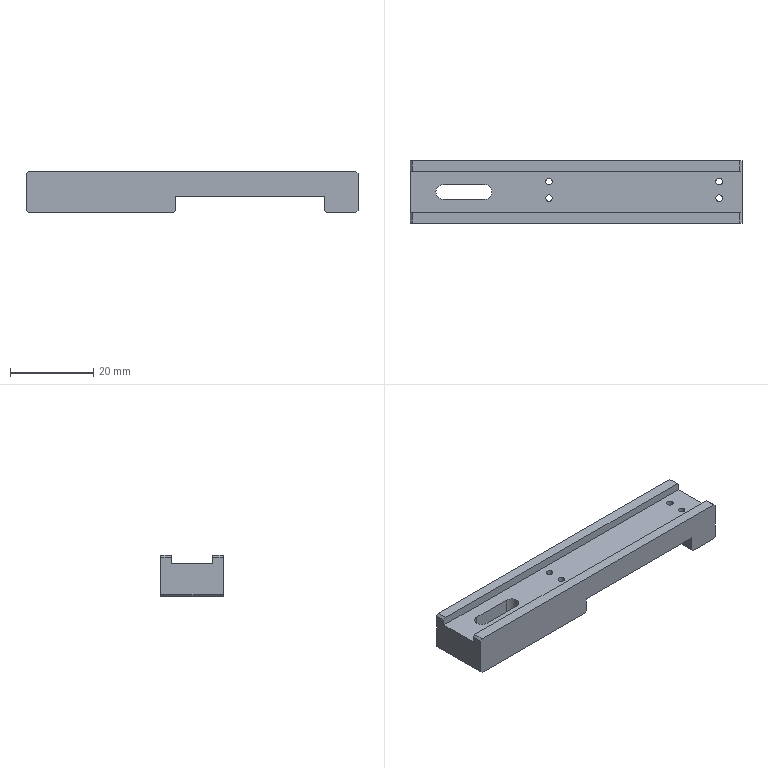Part | NX | 1 solid | 35 faces | box 80 x 15 x 10 mm | volume 7810 mm3 | plane 24 | cylinder 11 | commonest cylinder face diameters 1.6 x8 3.5 x3
STEP:
#1=CARTESIAN_POINT('',(-33.75,0.,-2.));
#2=VERTEX_POINT('',#1);
#3=CARTESIAN_POINT('',(-32.,1.75,-2.));
#4=VERTEX_POINT('',#3);
#5=CARTESIAN_POINT('',(-32.,0.,-2.));
#6=DIRECTION('',(0.,0.,-1.));
#7=DIRECTION('',(-1.,0.,0.));
#8=AXIS2_PLACEMENT_3D('',#5,#6,#7);
#9=CIRCLE('',#8,1.75);
#10=EDGE_CURVE('',#2,#4,#9,.T.);
#11=ORIENTED_EDGE('',*,*,#10,.F.);
#12=CARTESIAN_POINT('',(-33.75,0.,-10.));
#13=VERTEX_POINT('',#12);
#14=CARTESIAN_POINT('',(-33.75,0.,15.));
#15=DIRECTION('',(0.,0.,-1.));
#16=VECTOR('',#15,1000.);
#17=LINE('',#14,#16);
#18=EDGE_CURVE('',#2,#13,#17,.T.);
#19=ORIENTED_EDGE('',*,*,#18,.T.);
#20=CARTESIAN_POINT('',(-32.,1.75,-10.));
#21=VERTEX_POINT('',#20);
#22=CARTESIAN_POINT('',(-32.,0.,-10.));
#23=DIRECTION('',(0.,0.,-1.));
#24=DIRECTION('',(-1.,0.,0.));
#25=AXIS2_PLACEMENT_3D('',#22,#23,#24);
#26=CIRCLE('',#25,1.75);
#27=EDGE_CURVE('',#13,#21,#26,.T.);
#28=ORIENTED_EDGE('',*,*,#27,.T.);
#29=CARTESIAN_POINT('',(-32.,1.75,15.));
#30=DIRECTION('',(0.,0.,-1.));
#31=VECTOR('',#30,1000.);
#32=LINE('',#29,#31);
#33=EDGE_CURVE('',#4,#21,#32,.T.);
#34=ORIENTED_EDGE('',*,*,#33,.F.);
#35=EDGE_LOOP('',(#11,#19,#28,#34));
#36=FACE_BOUND('',#35,.T.);
#37=CARTESIAN_POINT('',(-32.,0.,15.));
#38=DIRECTION('',(0.,0.,-1.));
#39=DIRECTION('',(1.,0.,0.));
#40=AXIS2_PLACEMENT_3D('',#37,#38,#39);
#41=CYLINDRICAL_SURFACE('',#40,1.75);
#42=ADVANCED_FACE('',(#36),#41,.F.);
#43=CARTESIAN_POINT('',(33.7,2.5,-2.));
#44=VERTEX_POINT('',#43);
#45=CARTESIAN_POINT('',(35.3,2.5,-2.));
#46=VERTEX_POINT('',#45);
#47=CARTESIAN_POINT('',(34.5,2.5,-2.));
#48=DIRECTION('',(0.,0.,1.));
#49=DIRECTION('',(-1.,0.,0.));
#50=AXIS2_PLACEMENT_3D('',#47,#48,#49);
#51=CIRCLE('',#50,0.8);
#52=EDGE_CURVE('',#44,#46,#51,.T.);
#53=ORIENTED_EDGE('',*,*,#52,.T.);
#54=CARTESIAN_POINT('',(35.3,2.5,-10.));
#55=VERTEX_POINT('',#54);
#56=CARTESIAN_POINT('',(35.3,2.5,-10.));
#57=DIRECTION('',(0.,0.,-1.));
#58=VECTOR('',#57,1000.);
#59=LINE('',#56,#58);
#60=EDGE_CURVE('',#55,#46,#59,.F.);
#61=ORIENTED_EDGE('',*,*,#60,.F.);
#62=CARTESIAN_POINT('',(33.7,2.5,-10.));
#63=VERTEX_POINT('',#62);
#64=CARTESIAN_POINT('',(34.5,2.5,-10.));
#65=DIRECTION('',(0.,0.,-1.));
#66=DIRECTION('',(-1.,0.,0.));
#67=AXIS2_PLACEMENT_3D('',#64,#65,#66);
#68=CIRCLE('',#67,0.8);
#69=EDGE_CURVE('',#55,#63,#68,.T.);
#70=ORIENTED_EDGE('',*,*,#69,.T.);
#71=CARTESIAN_POINT('',(33.7,2.5,-10.));
#72=DIRECTION('',(0.,0.,-1.));
#73=VECTOR('',#72,1000.);
#74=LINE('',#71,#73);
#75=EDGE_CURVE('',#63,#44,#74,.F.);
#76=ORIENTED_EDGE('',*,*,#75,.T.);
#77=EDGE_LOOP('',(#53,#61,#70,#76));
#78=FACE_BOUND('',#77,.T.);
#79=CARTESIAN_POINT('',(34.5,2.5,-10.));
#80=DIRECTION('',(0.,0.,-1.));
#81=DIRECTION('',(1.,0.,0.));
#82=AXIS2_PLACEMENT_3D('',#79,#80,#81);
#83=CYLINDRICAL_SURFACE('',#82,0.8);
#84=ADVANCED_FACE('',(#78),#83,.F.);
#85=CARTESIAN_POINT('',(33.7,-1.5,-2.));
#86=VERTEX_POINT('',#85);
#87=CARTESIAN_POINT('',(35.3,-1.5,-2.));
#88=VERTEX_POINT('',#87);
#89=CARTESIAN_POINT('',(34.5,-1.5,-2.));
#90=DIRECTION('',(0.,0.,1.));
#91=DIRECTION('',(-1.,0.,0.));
#92=AXIS2_PLACEMENT_3D('',#89,#90,#91);
#93=CIRCLE('',#92,0.8);
#94=EDGE_CURVE('',#86,#88,#93,.T.);
#95=ORIENTED_EDGE('',*,*,#94,.T.);
#96=CARTESIAN_POINT('',(35.3,-1.5,-10.));
#97=VERTEX_POINT('',#96);
#98=CARTESIAN_POINT('',(35.3,-1.5,-10.));
#99=DIRECTION('',(0.,0.,-1.));
#100=VECTOR('',#99,1000.);
#101=LINE('',#98,#100);
#102=EDGE_CURVE('',#97,#88,#101,.F.);
#103=ORIENTED_EDGE('',*,*,#102,.F.);
#104=CARTESIAN_POINT('',(33.7,-1.5,-10.));
#105=VERTEX_POINT('',#104);
#106=CARTESIAN_POINT('',(34.5,-1.5,-10.));
#107=DIRECTION('',(0.,0.,-1.));
#108=DIRECTION('',(-1.,0.,0.));
#109=AXIS2_PLACEMENT_3D('',#106,#107,#108);
#110=CIRCLE('',#109,0.8);
#111=EDGE_CURVE('',#97,#105,#110,.T.);
#112=ORIENTED_EDGE('',*,*,#111,.T.);
#113=CARTESIAN_POINT('',(33.7,-1.5,-10.));
#114=DIRECTION('',(0.,0.,-1.));
#115=VECTOR('',#114,1000.);
#116=LINE('',#113,#115);
#117=EDGE_CURVE('',#105,#86,#116,.F.);
#118=ORIENTED_EDGE('',*,*,#117,.T.);
#119=EDGE_LOOP('',(#95,#103,#112,#118));
#120=FACE_BOUND('',#119,.T.);
#121=CARTESIAN_POINT('',(34.5,-1.5,-10.));
#122=DIRECTION('',(0.,0.,-1.));
#123=DIRECTION('',(1.,0.,0.));
#124=AXIS2_PLACEMENT_3D('',#121,#122,#123);
#125=CYLINDRICAL_SURFACE('',#124,0.8);
#126=ADVANCED_FACE('',(#120),#125,.F.);
#127=CARTESIAN_POINT('',(-7.3,-1.5,-2.));
#128=VERTEX_POINT('',#127);
#129=CARTESIAN_POINT('',(-5.7,-1.5,-2.));
#130=VERTEX_POINT('',#129);
#131=CARTESIAN_POINT('',(-6.5,-1.5,-2.));
#132=DIRECTION('',(0.,0.,1.));
#133=DIRECTION('',(-1.,0.,0.));
#134=AXIS2_PLACEMENT_3D('',#131,#132,#133);
#135=CIRCLE('',#134,0.8);
#136=EDGE_CURVE('',#128,#130,#135,.T.);
#137=ORIENTED_EDGE('',*,*,#136,.T.);
#138=CARTESIAN_POINT('',(-5.7,-1.5,-10.));
#139=VERTEX_POINT('',#138);
#140=CARTESIAN_POINT('',(-5.7,-1.5,-10.));
#141=DIRECTION('',(0.,0.,-1.));
#142=VECTOR('',#141,1000.);
#143=LINE('',#140,#142);
#144=EDGE_CURVE('',#139,#130,#143,.F.);
#145=ORIENTED_EDGE('',*,*,#144,.F.);
#146=CARTESIAN_POINT('',(-7.3,-1.5,-10.));
#147=VERTEX_POINT('',#146);
#148=CARTESIAN_POINT('',(-6.5,-1.5,-10.));
#149=DIRECTION('',(0.,0.,-1.));
#150=DIRECTION('',(-1.,0.,0.));
#151=AXIS2_PLACEMENT_3D('',#148,#149,#150);
#152=CIRCLE('',#151,0.8);
#153=EDGE_CURVE('',#139,#147,#152,.T.);
#154=ORIENTED_EDGE('',*,*,#153,.T.);
#155=CARTESIAN_POINT('',(-7.3,-1.5,-10.));
#156=DIRECTION('',(0.,0.,-1.));
#157=VECTOR('',#156,1000.);
#158=LINE('',#155,#157);
#159=EDGE_CURVE('',#147,#128,#158,.F.);
#160=ORIENTED_EDGE('',*,*,#159,.T.);
#161=EDGE_LOOP('',(#137,#145,#154,#160));
#162=FACE_BOUND('',#161,.T.);
#163=CARTESIAN_POINT('',(-6.5,-1.5,-10.));
#164=DIRECTION('',(0.,0.,-1.));
#165=DIRECTION('',(1.,0.,0.));
#166=AXIS2_PLACEMENT_3D('',#163,#164,#165);
#167=CYLINDRICAL_SURFACE('',#166,0.8);
#168=ADVANCED_FACE('',(#162),#167,.F.);
#169=CARTESIAN_POINT('',(-7.3,2.5,-2.));
#170=VERTEX_POINT('',#169);
#171=CARTESIAN_POINT('',(-5.7,2.5,-2.));
#172=VERTEX_POINT('',#171);
#173=CARTESIAN_POINT('',(-6.5,2.5,-2.));
#174=DIRECTION('',(0.,0.,1.));
#175=DIRECTION('',(-1.,0.,0.));
#176=AXIS2_PLACEMENT_3D('',#173,#174,#175);
#177=CIRCLE('',#176,0.8);
#178=EDGE_CURVE('',#170,#172,#177,.T.);
#179=ORIENTED_EDGE('',*,*,#178,.T.);
#180=CARTESIAN_POINT('',(-5.7,2.5,-10.));
#181=VERTEX_POINT('',#180);
#182=CARTESIAN_POINT('',(-5.7,2.5,-10.));
#183=DIRECTION('',(0.,0.,-1.));
#184=VECTOR('',#183,1000.);
#185=LINE('',#182,#184);
#186=EDGE_CURVE('',#181,#172,#185,.F.);
#187=ORIENTED_EDGE('',*,*,#186,.F.);
#188=CARTESIAN_POINT('',(-7.3,2.5,-10.));
#189=VERTEX_POINT('',#188);
#190=CARTESIAN_POINT('',(-6.5,2.5,-10.));
#191=DIRECTION('',(0.,0.,-1.));
#192=DIRECTION('',(-1.,0.,0.));
#193=AXIS2_PLACEMENT_3D('',#190,#191,#192);
#194=CIRCLE('',#193,0.8);
#195=EDGE_CURVE('',#181,#189,#194,.T.);
#196=ORIENTED_EDGE('',*,*,#195,.T.);
#197=CARTESIAN_POINT('',(-7.3,2.5,-10.));
#198=DIRECTION('',(0.,0.,-1.));
#199=VECTOR('',#198,1000.);
#200=LINE('',#197,#199);
#201=EDGE_CURVE('',#189,#170,#200,.F.);
#202=ORIENTED_EDGE('',*,*,#201,.T.);
#203=EDGE_LOOP('',(#179,#187,#196,#202));
#204=FACE_BOUND('',#203,.T.);
#205=CARTESIAN_POINT('',(-6.5,2.5,-10.));
#206=DIRECTION('',(0.,0.,-1.));
#207=DIRECTION('',(1.,0.,0.));
#208=AXIS2_PLACEMENT_3D('',#205,#206,#207);
#209=CYLINDRICAL_SURFACE('',#208,0.8);
#210=ADVANCED_FACE('',(#204),#209,.F.);
#211=CARTESIAN_POINT('',(39.5,-7.5,0.));
#212=VERTEX_POINT('',#211);
#213=CARTESIAN_POINT('',(39.5,-5.,0.));
#214=VERTEX_POINT('',#213);
#215=CARTESIAN_POINT('',(39.5,0.,0.));
#216=DIRECTION('',(0.,1.,0.));
#217=VECTOR('',#216,1000.);
#218=LINE('',#215,#217);
#219=EDGE_CURVE('',#212,#214,#218,.T.);
#220=ORIENTED_EDGE('',*,*,#219,.T.);
#221=CARTESIAN_POINT('',(-39.5,-5.,0.));
#222=VERTEX_POINT('',#221);
#223=CARTESIAN_POINT('',(49.,-5.,0.));
#224=DIRECTION('',(-1.,0.,0.));
#225=VECTOR('',#224,1000.);
#226=LINE('',#223,#225);
#227=EDGE_CURVE('',#214,#222,#226,.T.);
#228=ORIENTED_EDGE('',*,*,#227,.T.);
#229=CARTESIAN_POINT('',(-39.5,-7.5,0.));
#230=VERTEX_POINT('',#229);
#231=CARTESIAN_POINT('',(-39.5,0.,0.));
#232=DIRECTION('',(0.,-1.,0.));
#233=VECTOR('',#232,1000.);
#234=LINE('',#231,#233);
#235=EDGE_CURVE('',#222,#230,#234,.T.);
#236=ORIENTED_EDGE('',*,*,#235,.T.);
#237=CARTESIAN_POINT('',(40.,-7.5,0.));
#238=DIRECTION('',(-1.,0.,0.));
#239=VECTOR('',#238,1000.);
#240=LINE('',#237,#239);
#241=EDGE_CURVE('',#212,#230,#240,.T.);
#242=ORIENTED_EDGE('',*,*,#241,.F.);
#243=EDGE_LOOP('',(#220,#228,#236,#242));
#244=FACE_BOUND('',#243,.T.);
#245=CARTESIAN_POINT('',(0.,0.,0.));
#246=DIRECTION('',(0.,0.,-1.));
#247=DIRECTION('',(1.,0.,0.));
#248=AXIS2_PLACEMENT_3D('',#245,#246,#247);
#249=PLANE('',#248);
#250=ADVANCED_FACE('',(#244),#249,.F.);
#251=CARTESIAN_POINT('',(-40.,-5.,-0.5));
#252=VERTEX_POINT('',#251);
#253=CARTESIAN_POINT('',(-40.,-5.,-0.5));
#254=DIRECTION('',(0.7071,0.,0.7071));
#255=VECTOR('',#254,1000.);
#256=LINE('',#253,#255);
#257=EDGE_CURVE('',#252,#222,#256,.T.);
#258=ORIENTED_EDGE('',*,*,#257,.F.);
#259=CARTESIAN_POINT('',(-40.,-7.5,-0.5));
#260=VERTEX_POINT('',#259);
#261=CARTESIAN_POINT('',(-40.,-7.5,-0.5));
#262=DIRECTION('',(0.,1.,0.));
#263=VECTOR('',#262,1000.);
#264=LINE('',#261,#263);
#265=EDGE_CURVE('',#260,#252,#264,.T.);
#266=ORIENTED_EDGE('',*,*,#265,.F.);
#267=CARTESIAN_POINT('',(-40.,-7.5,-0.5));
#268=DIRECTION('',(-0.7071,0.,-0.7071));
#269=VECTOR('',#268,1000.);
#270=LINE('',#267,#269);
#271=EDGE_CURVE('',#230,#260,#270,.T.);
#272=ORIENTED_EDGE('',*,*,#271,.F.);
#273=ORIENTED_EDGE('',*,*,#235,.F.);
#274=EDGE_LOOP('',(#258,#266,#272,#273));
#275=FACE_BOUND('',#274,.T.);
#276=CARTESIAN_POINT('',(-40.,-7.5,-0.5));
#277=DIRECTION('',(0.7071,0.,-0.7071));
#278=DIRECTION('',(0.,-1.,0.));
#279=AXIS2_PLACEMENT_3D('',#276,#277,#278);
#280=PLANE('',#279);
#281=ADVANCED_FACE('',(#275),#280,.F.);
#282=CARTESIAN_POINT('',(40.,-5.,-0.5));
#283=VERTEX_POINT('',#282);
#284=CARTESIAN_POINT('',(40.,-5.,-0.5));
#285=DIRECTION('',(0.7071,0.,-0.7071));
#286=VECTOR('',#285,1000.);
#287=LINE('',#284,#286);
#288=EDGE_CURVE('',#214,#283,#287,.T.);
#289=ORIENTED_EDGE('',*,*,#288,.F.);
#290=ORIENTED_EDGE('',*,*,#219,.F.);
#291=CARTESIAN_POINT('',(40.,-7.5,-0.5));
#292=VERTEX_POINT('',#291);
#293=CARTESIAN_POINT('',(40.,-7.5,-0.5));
#294=DIRECTION('',(-0.7071,0.,0.7071));
#295=VECTOR('',#294,1000.);
#296=LINE('',#293,#295);
#297=EDGE_CURVE('',#292,#212,#296,.T.);
#298=ORIENTED_EDGE('',*,*,#297,.F.);
#299=CARTESIAN_POINT('',(40.,-7.5,-0.5));
#300=DIRECTION('',(0.,-1.,0.));
#301=VECTOR('',#300,1000.);
#302=LINE('',#299,#301);
#303=EDGE_CURVE('',#283,#292,#302,.T.);
#304=ORIENTED_EDGE('',*,*,#303,.F.);
#305=EDGE_LOOP('',(#289,#290,#298,#304));
#306=FACE_BOUND('',#305,.T.);
#307=CARTESIAN_POINT('',(40.,-7.5,-0.5));
#308=DIRECTION('',(-0.7071,0.,-0.7071));
#309=DIRECTION('',(0.,1.,0.));
#310=AXIS2_PLACEMENT_3D('',#307,#308,#309);
#311=PLANE('',#310);
#312=ADVANCED_FACE('',(#306),#311,.F.);
#313=CARTESIAN_POINT('',(34.5,2.5,-10.));
#314=DIRECTION('',(0.,0.,-1.));
#315=DIRECTION('',(-1.,0.,0.));
#316=AXIS2_PLACEMENT_3D('',#313,#314,#315);
#317=CIRCLE('',#316,0.8);
#318=EDGE_CURVE('',#63,#55,#317,.T.);
#319=ORIENTED_EDGE('',*,*,#318,.F.);
#320=ORIENTED_EDGE('',*,*,#69,.F.);
#321=EDGE_LOOP('',(#319,#320));
#322=FACE_BOUND('',#321,.T.);
#323=CARTESIAN_POINT('',(34.5,-1.5,-10.));
#324=DIRECTION('',(0.,0.,-1.));
#325=DIRECTION('',(-1.,0.,0.));
#326=AXIS2_PLACEMENT_3D('',#323,#324,#325);
#327=CIRCLE('',#326,0.8);
#328=EDGE_CURVE('',#105,#97,#327,.T.);
#329=ORIENTED_EDGE('',*,*,#328,.F.);
#330=ORIENTED_EDGE('',*,*,#111,.F.);
#331=EDGE_LOOP('',(#329,#330));
#332=FACE_BOUND('',#331,.T.);
#333=CARTESIAN_POINT('',(32.5,7.5,-10.));
#334=VERTEX_POINT('',#333);
#335=CARTESIAN_POINT('',(39.5,7.5,-10.));
#336=VERTEX_POINT('',#335);
#337=CARTESIAN_POINT('',(40.,7.5,-10.));
#338=DIRECTION('',(1.,0.,0.));
#339=VECTOR('',#338,1000.);
#340=LINE('',#337,#339);
#341=EDGE_CURVE('',#334,#336,#340,.T.);
#342=ORIENTED_EDGE('',*,*,#341,.T.);
#343=CARTESIAN_POINT('',(39.5,-7.5,-10.));
#344=VERTEX_POINT('',#343);
#345=CARTESIAN_POINT('',(39.5,-7.5,-10.));
#346=DIRECTION('',(0.,-1.,0.));
#347=VECTOR('',#346,1000.);
#348=LINE('',#345,#347);
#349=EDGE_CURVE('',#336,#344,#348,.T.);
#350=ORIENTED_EDGE('',*,*,#349,.T.);
#351=CARTESIAN_POINT('',(32.5,-7.5,-10.));
#352=VERTEX_POINT('',#351);
#353=CARTESIAN_POINT('',(40.,-7.5,-10.));
#354=DIRECTION('',(-1.,0.,0.));
#355=VECTOR('',#354,1000.);
#356=LINE('',#353,#355);
#357=EDGE_CURVE('',#344,#352,#356,.T.);
#358=ORIENTED_EDGE('',*,*,#357,.T.);
#359=CARTESIAN_POINT('',(32.5,7.5,-10.));
#360=DIRECTION('',(0.,1.,0.));
#361=VECTOR('',#360,1000.);
#362=LINE('',#359,#361);
#363=EDGE_CURVE('',#352,#334,#362,.T.);
#364=ORIENTED_EDGE('',*,*,#363,.T.);
#365=EDGE_LOOP('',(#342,#350,#358,#364));
#366=FACE_BOUND('',#365,.T.);
#367=CARTESIAN_POINT('',(0.,0.,-10.));
#368=DIRECTION('',(0.,0.,-1.));
#369=DIRECTION('',(1.,0.,0.));
#370=AXIS2_PLACEMENT_3D('',#367,#368,#369);
#371=PLANE('',#370);
#372=ADVANCED_FACE('',(#322,#332,#366),#371,.T.);
#373=CARTESIAN_POINT('',(-40.,7.5,-9.5));
#374=VERTEX_POINT('',#373);
#375=CARTESIAN_POINT('',(-40.,7.5,-0.5));
#376=VERTEX_POINT('',#375);
#377=CARTESIAN_POINT('',(-40.,7.5,-10.));
#378=DIRECTION('',(0.,0.,1.));
#379=VECTOR('',#378,1000.);
#380=LINE('',#377,#379);
#381=EDGE_CURVE('',#374,#376,#380,.T.);
#382=ORIENTED_EDGE('',*,*,#381,.T.);
#383=CARTESIAN_POINT('',(-39.5,7.5,0.));
#384=VERTEX_POINT('',#383);
#385=CARTESIAN_POINT('',(-40.,7.5,-0.5));
#386=DIRECTION('',(0.7071,0.,0.7071));
#387=VECTOR('',#386,1000.);
#388=LINE('',#385,#387);
#389=EDGE_CURVE('',#376,#384,#388,.T.);
#390=ORIENTED_EDGE('',*,*,#389,.T.);
#391=CARTESIAN_POINT('',(39.5,7.5,0.));
#392=VERTEX_POINT('',#391);
#393=CARTESIAN_POINT('',(40.,7.5,0.));
#394=DIRECTION('',(1.,0.,0.));
#395=VECTOR('',#394,1000.);
#396=LINE('',#393,#395);
#397=EDGE_CURVE('',#384,#392,#396,.T.);
#398=ORIENTED_EDGE('',*,*,#397,.T.);
#399=CARTESIAN_POINT('',(40.,7.5,-0.5));
#400=VERTEX_POINT('',#399);
#401=CARTESIAN_POINT('',(40.,7.5,-0.5));
#402=DIRECTION('',(0.7071,0.,-0.7071));
#403=VECTOR('',#402,1000.);
#404=LINE('',#401,#403);
#405=EDGE_CURVE('',#392,#400,#404,.T.);
#406=ORIENTED_EDGE('',*,*,#405,.T.);
#407=CARTESIAN_POINT('',(40.,7.5,-9.5));
#408=VERTEX_POINT('',#407);
#409=CARTESIAN_POINT('',(40.,7.5,-10.));
#410=DIRECTION('',(0.,0.,1.));
#411=VECTOR('',#410,1000.);
#412=LINE('',#409,#411);
#413=EDGE_CURVE('',#408,#400,#412,.T.);
#414=ORIENTED_EDGE('',*,*,#413,.F.);
#415=CARTESIAN_POINT('',(39.5,7.5,-10.));
#416=DIRECTION('',(-0.7071,0.,-0.7071));
#417=VECTOR('',#416,1000.);
#418=LINE('',#415,#417);
#419=EDGE_CURVE('',#408,#336,#418,.T.);
#420=ORIENTED_EDGE('',*,*,#419,.T.);
#421=ORIENTED_EDGE('',*,*,#341,.F.);
#422=CARTESIAN_POINT('',(32.,7.5,-9.5));
#423=VERTEX_POINT('',#422);
#424=CARTESIAN_POINT('',(32.5,7.5,-10.));
#425=DIRECTION('',(-0.7071,0.,0.7071));
#426=VECTOR('',#425,1000.);
#427=LINE('',#424,#426);
#428=EDGE_CURVE('',#334,#423,#427,.T.);
#429=ORIENTED_EDGE('',*,*,#428,.T.);
#430=CARTESIAN_POINT('',(32.,7.5,-6.));
#431=VERTEX_POINT('',#430);
#432=CARTESIAN_POINT('',(32.,7.5,-10.));
#433=DIRECTION('',(0.,0.,-1.));
#434=VECTOR('',#433,1000.);
#435=LINE('',#432,#434);
#436=EDGE_CURVE('',#431,#423,#435,.T.);
#437=ORIENTED_EDGE('',*,*,#436,.F.);
#438=CARTESIAN_POINT('',(-4.,7.5,-6.));
#439=VERTEX_POINT('',#438);
#440=CARTESIAN_POINT('',(32.,7.5,-6.));
#441=DIRECTION('',(1.,0.,0.));
#442=VECTOR('',#441,1000.);
#443=LINE('',#440,#442);
#444=EDGE_CURVE('',#439,#431,#443,.T.);
#445=ORIENTED_EDGE('',*,*,#444,.F.);
#446=CARTESIAN_POINT('',(-4.,7.5,-9.5));
#447=VERTEX_POINT('',#446);
#448=CARTESIAN_POINT('',(-4.,7.5,-10.));
#449=DIRECTION('',(0.,0.,1.));
#450=VECTOR('',#449,1000.);
#451=LINE('',#448,#450);
#452=EDGE_CURVE('',#447,#439,#451,.T.);
#453=ORIENTED_EDGE('',*,*,#452,.F.);
#454=CARTESIAN_POINT('',(-4.5,7.5,-10.));
#455=VERTEX_POINT('',#454);
#456=CARTESIAN_POINT('',(-4.,7.5,-9.5));
#457=DIRECTION('',(-0.7071,0.,-0.7071));
#458=VECTOR('',#457,1000.);
#459=LINE('',#456,#458);
#460=EDGE_CURVE('',#447,#455,#459,.T.);
#461=ORIENTED_EDGE('',*,*,#460,.T.);
#462=CARTESIAN_POINT('',(-39.5,7.5,-10.));
#463=VERTEX_POINT('',#462);
#464=CARTESIAN_POINT('',(40.,7.5,-10.));
#465=DIRECTION('',(1.,0.,0.));
#466=VECTOR('',#465,1000.);
#467=LINE('',#464,#466);
#468=EDGE_CURVE('',#463,#455,#467,.T.);
#469=ORIENTED_EDGE('',*,*,#468,.F.);
#470=CARTESIAN_POINT('',(-39.5,7.5,-10.));
#471=DIRECTION('',(-0.7071,0.,0.7071));
#472=VECTOR('',#471,1000.);
#473=LINE('',#470,#472);
#474=EDGE_CURVE('',#463,#374,#473,.T.);
#475=ORIENTED_EDGE('',*,*,#474,.T.);
#476=EDGE_LOOP('',(#382,#390,#398,#406,#414,#420,#421,#429,#437,#445,#453,#461,#469,#475));
#477=FACE_BOUND('',#476,.T.);
#478=CARTESIAN_POINT('',(40.,7.5,-10.));
#479=DIRECTION('',(0.,-1.,0.));
#480=DIRECTION('',(1.,0.,0.));
#481=AXIS2_PLACEMENT_3D('',#478,#479,#480);
#482=PLANE('',#481);
#483=ADVANCED_FACE('',(#477),#482,.F.);
#484=CARTESIAN_POINT('',(40.,5.,-2.));
#485=VERTEX_POINT('',#484);
#486=CARTESIAN_POINT('',(40.,-5.,-2.));
#487=VERTEX_POINT('',#486);
#488=CARTESIAN_POINT('',(40.,-7.5,-2.));
#489=DIRECTION('',(0.,-1.,0.));
#490=VECTOR('',#489,1000.);
#491=LINE('',#488,#490);
#492=EDGE_CURVE('',#485,#487,#491,.T.);
#493=ORIENTED_EDGE('',*,*,#492,.T.);
#494=CARTESIAN_POINT('',(40.,-5.,-10.));
#495=DIRECTION('',(0.,0.,1.));
#496=VECTOR('',#495,1000.);
#497=LINE('',#494,#496);
#498=EDGE_CURVE('',#487,#283,#497,.T.);
#499=ORIENTED_EDGE('',*,*,#498,.T.);
#500=ORIENTED_EDGE('',*,*,#303,.T.);
#501=CARTESIAN_POINT('',(40.,-7.5,-9.5));
#502=VERTEX_POINT('',#501);
#503=CARTESIAN_POINT('',(40.,-7.5,-10.));
#504=DIRECTION('',(0.,0.,1.));
#505=VECTOR('',#504,1000.);
#506=LINE('',#503,#505);
#507=EDGE_CURVE('',#502,#292,#506,.T.);
#508=ORIENTED_EDGE('',*,*,#507,.F.);
#509=CARTESIAN_POINT('',(40.,7.5,-9.5));
#510=DIRECTION('',(0.,1.,0.));
#511=VECTOR('',#510,1000.);
#512=LINE('',#509,#511);
#513=EDGE_CURVE('',#502,#408,#512,.T.);
#514=ORIENTED_EDGE('',*,*,#513,.T.);
#515=ORIENTED_EDGE('',*,*,#413,.T.);
#516=CARTESIAN_POINT('',(40.,5.,-0.5));
#517=VERTEX_POINT('',#516);
#518=CARTESIAN_POINT('',(40.,-7.5,-0.5));
#519=DIRECTION('',(0.,-1.,0.));
#520=VECTOR('',#519,1000.);
#521=LINE('',#518,#520);
#522=EDGE_CURVE('',#400,#517,#521,.T.);
#523=ORIENTED_EDGE('',*,*,#522,.T.);
#524=CARTESIAN_POINT('',(40.,5.,-10.));
#525=DIRECTION('',(0.,0.,-1.));
#526=VECTOR('',#525,1000.);
#527=LINE('',#524,#526);
#528=EDGE_CURVE('',#517,#485,#527,.T.);
#529=ORIENTED_EDGE('',*,*,#528,.T.);
#530=EDGE_LOOP('',(#493,#499,#500,#508,#514,#515,#523,#529));
#531=FACE_BOUND('',#530,.T.);
#532=CARTESIAN_POINT('',(40.,-7.5,-10.));
#533=DIRECTION('',(-1.,0.,0.));
#534=DIRECTION('',(0.,-1.,0.));
#535=AXIS2_PLACEMENT_3D('',#532,#533,#534);
#536=PLANE('',#535);
#537=ADVANCED_FACE('',(#531),#536,.F.);
#538=ORIENTED_EDGE('',*,*,#241,.T.);
#539=ORIENTED_EDGE('',*,*,#271,.T.);
#540=CARTESIAN_POINT('',(-40.,-7.5,-9.5));
#541=VERTEX_POINT('',#540);
#542=CARTESIAN_POINT('',(-40.,-7.5,-10.));
#543=DIRECTION('',(0.,0.,1.));
#544=VECTOR('',#543,1000.);
#545=LINE('',#542,#544);
#546=EDGE_CURVE('',#541,#260,#545,.T.);
#547=ORIENTED_EDGE('',*,*,#546,.F.);
#548=CARTESIAN_POINT('',(-39.5,-7.5,-10.));
#549=VERTEX_POINT('',#548);
#550=CARTESIAN_POINT('',(-39.5,-7.5,-10.));
#551=DIRECTION('',(0.7071,0.,-0.7071));
#552=VECTOR('',#551,1000.);
#553=LINE('',#550,#552);
#554=EDGE_CURVE('',#541,#549,#553,.T.);
#555=ORIENTED_EDGE('',*,*,#554,.T.);
#556=CARTESIAN_POINT('',(-4.5,-7.5,-10.));
#557=VERTEX_POINT('',#556);
#558=CARTESIAN_POINT('',(40.,-7.5,-10.));
#559=DIRECTION('',(-1.,0.,0.));
#560=VECTOR('',#559,1000.);
#561=LINE('',#558,#560);
#562=EDGE_CURVE('',#557,#549,#561,.T.);
#563=ORIENTED_EDGE('',*,*,#562,.F.);
#564=CARTESIAN_POINT('',(-4.,-7.5,-9.5));
#565=VERTEX_POINT('',#564);
#566=CARTESIAN_POINT('',(-4.,-7.5,-9.5));
#567=DIRECTION('',(0.7071,0.,0.7071));
#568=VECTOR('',#567,1000.);
#569=LINE('',#566,#568);
#570=EDGE_CURVE('',#557,#565,#569,.T.);
#571=ORIENTED_EDGE('',*,*,#570,.T.);
#572=CARTESIAN_POINT('',(-4.,-7.5,-6.));
#573=VERTEX_POINT('',#572);
#574=CARTESIAN_POINT('',(-4.,-7.5,-10.));
#575=DIRECTION('',(0.,0.,1.));
#576=VECTOR('',#575,1000.);
#577=LINE('',#574,#576);
#578=EDGE_CURVE('',#565,#573,#577,.T.);
#579=ORIENTED_EDGE('',*,*,#578,.T.);
#580=CARTESIAN_POINT('',(32.,-7.5,-6.));
#581=VERTEX_POINT('',#580);
#582=CARTESIAN_POINT('',(32.,-7.5,-6.));
#583=DIRECTION('',(1.,0.,0.));
#584=VECTOR('',#583,1000.);
#585=LINE('',#582,#584);
#586=EDGE_CURVE('',#573,#581,#585,.T.);
#587=ORIENTED_EDGE('',*,*,#586,.T.);
#588=CARTESIAN_POINT('',(32.,-7.5,-9.5));
#589=VERTEX_POINT('',#588);
#590=CARTESIAN_POINT('',(32.,-7.5,-10.));
#591=DIRECTION('',(0.,0.,-1.));
#592=VECTOR('',#591,1000.);
#593=LINE('',#590,#592);
#594=EDGE_CURVE('',#581,#589,#593,.T.);
#595=ORIENTED_EDGE('',*,*,#594,.T.);
#596=CARTESIAN_POINT('',(32.5,-7.5,-10.));
#597=DIRECTION('',(0.7071,0.,-0.7071));
#598=VECTOR('',#597,1000.);
#599=LINE('',#596,#598);
#600=EDGE_CURVE('',#589,#352,#599,.T.);
#601=ORIENTED_EDGE('',*,*,#600,.T.);
#602=ORIENTED_EDGE('',*,*,#357,.F.);
#603=CARTESIAN_POINT('',(39.5,-7.5,-10.));
#604=DIRECTION('',(0.7071,0.,0.7071));
#605=VECTOR('',#604,1000.);
#606=LINE('',#603,#605);
#607=EDGE_CURVE('',#344,#502,#606,.T.);
#608=ORIENTED_EDGE('',*,*,#607,.T.);
#609=ORIENTED_EDGE('',*,*,#507,.T.);
#610=ORIENTED_EDGE('',*,*,#297,.T.);
#611=EDGE_LOOP('',(#538,#539,#547,#555,#563,#571,#579,#587,#595,#601,#602,#608,#609,#610));
#612=FACE_BOUND('',#611,.T.);
#613=CARTESIAN_POINT('',(40.,-7.5,-10.));
#614=DIRECTION('',(0.,1.,0.));
#615=DIRECTION('',(-1.,0.,0.));
#616=AXIS2_PLACEMENT_3D('',#613,#614,#615);
#617=PLANE('',#616);
#618=ADVANCED_FACE('',(#612),#617,.F.);
#619=ORIENTED_EDGE('',*,*,#265,.T.);
#620=CARTESIAN_POINT('',(-40.,-5.,-2.));
#621=VERTEX_POINT('',#620);
#622=CARTESIAN_POINT('',(-40.,-5.,0.));
#623=DIRECTION('',(0.,0.,1.));
#624=VECTOR('',#623,1000.);
#625=LINE('',#622,#624);
#626=EDGE_CURVE('',#621,#252,#625,.T.);
#627=ORIENTED_EDGE('',*,*,#626,.F.);
#628=CARTESIAN_POINT('',(-40.,5.,-2.));
#629=VERTEX_POINT('',#628);
#630=CARTESIAN_POINT('',(-40.,-5.,-2.));
#631=DIRECTION('',(0.,-1.,0.));
#632=VECTOR('',#631,1000.);
#633=LINE('',#630,#632);
#634=EDGE_CURVE('',#629,#621,#633,.T.);
#635=ORIENTED_EDGE('',*,*,#634,.F.);
#636=CARTESIAN_POINT('',(-40.,5.,-0.5));
#637=VERTEX_POINT('',#636);
#638=CARTESIAN_POINT('',(-40.,5.,0.));
#639=DIRECTION('',(0.,0.,-1.));
#640=VECTOR('',#639,1000.);
#641=LINE('',#638,#640);
#642=EDGE_CURVE('',#637,#629,#641,.T.);
#643=ORIENTED_EDGE('',*,*,#642,.F.);
#644=CARTESIAN_POINT('',(-40.,-7.5,-0.5));
#645=DIRECTION('',(0.,1.,0.));
#646=VECTOR('',#645,1000.);
#647=LINE('',#644,#646);
#648=EDGE_CURVE('',#637,#376,#647,.T.);
#649=ORIENTED_EDGE('',*,*,#648,.T.);
#650=ORIENTED_EDGE('',*,*,#381,.F.);
#651=CARTESIAN_POINT('',(-40.,-7.5,-9.5));
#652=DIRECTION('',(0.,-1.,0.));
#653=VECTOR('',#652,1000.);
#654=LINE('',#651,#653);
#655=EDGE_CURVE('',#374,#541,#654,.T.);
#656=ORIENTED_EDGE('',*,*,#655,.T.);
#657=ORIENTED_EDGE('',*,*,#546,.T.);
#658=EDGE_LOOP('',(#619,#627,#635,#643,#649,#650,#656,#657));
#659=FACE_BOUND('',#658,.T.);
#660=CARTESIAN_POINT('',(-40.,-7.5,-10.));
#661=DIRECTION('',(1.,0.,0.));
#662=DIRECTION('',(0.,1.,0.));
#663=AXIS2_PLACEMENT_3D('',#660,#661,#662);
#664=PLANE('',#663);
#665=ADVANCED_FACE('',(#659),#664,.F.);
#666=CARTESIAN_POINT('',(-22.,1.75,-10.));
#667=VERTEX_POINT('',#666);
#668=CARTESIAN_POINT('',(-22.,-1.75,-10.));
#669=VERTEX_POINT('',#668);
#670=CARTESIAN_POINT('',(-22.,0.,-10.));
#671=DIRECTION('',(0.,0.,-1.));
#672=DIRECTION('',(-1.,0.,0.));
#673=AXIS2_PLACEMENT_3D('',#670,#671,#672);
#674=CIRCLE('',#673,1.75);
#675=EDGE_CURVE('',#667,#669,#674,.T.);
#676=ORIENTED_EDGE('',*,*,#675,.F.);
#677=CARTESIAN_POINT('',(-22.,1.75,-10.));
#678=DIRECTION('',(1.,0.,0.));
#679=VECTOR('',#678,1000.);
#680=LINE('',#677,#679);
#681=EDGE_CURVE('',#21,#667,#680,.T.);
#682=ORIENTED_EDGE('',*,*,#681,.F.);
#683=ORIENTED_EDGE('',*,*,#27,.F.);
#684=CARTESIAN_POINT('',(-32.,-1.75,-10.));
#685=VERTEX_POINT('',#684);
#686=CARTESIAN_POINT('',(-32.,0.,-10.));
#687=DIRECTION('',(0.,0.,-1.));
#688=DIRECTION('',(-1.,0.,0.));
#689=AXIS2_PLACEMENT_3D('',#686,#687,#688);
#690=CIRCLE('',#689,1.75);
#691=EDGE_CURVE('',#685,#13,#690,.T.);
#692=ORIENTED_EDGE('',*,*,#691,.F.);
#693=CARTESIAN_POINT('',(-22.,-1.75,-10.));
#694=DIRECTION('',(-1.,0.,0.));
#695=VECTOR('',#694,1000.);
#696=LINE('',#693,#695);
#697=EDGE_CURVE('',#669,#685,#696,.T.);
#698=ORIENTED_EDGE('',*,*,#697,.F.);
#699=EDGE_LOOP('',(#676,#682,#683,#692,#698));
#700=FACE_BOUND('',#699,.T.);
#701=CARTESIAN_POINT('',(-6.5,-1.5,-10.));
#702=DIRECTION('',(0.,0.,-1.));
#703=DIRECTION('',(-1.,0.,0.));
#704=AXIS2_PLACEMENT_3D('',#701,#702,#703);
#705=CIRCLE('',#704,0.8);
#706=EDGE_CURVE('',#147,#139,#705,.T.);
#707=ORIENTED_EDGE('',*,*,#706,.F.);
#708=ORIENTED_EDGE('',*,*,#153,.F.);
#709=EDGE_LOOP('',(#707,#708));
#710=FACE_BOUND('',#709,.T.);
#711=CARTESIAN_POINT('',(-6.5,2.5,-10.));
#712=DIRECTION('',(0.,0.,-1.));
#713=DIRECTION('',(-1.,0.,0.));
#714=AXIS2_PLACEMENT_3D('',#711,#712,#713);
#715=CIRCLE('',#714,0.8);
#716=EDGE_CURVE('',#189,#181,#715,.T.);
#717=ORIENTED_EDGE('',*,*,#716,.F.);
#718=ORIENTED_EDGE('',*,*,#195,.F.);
#719=EDGE_LOOP('',(#717,#718));
#720=FACE_BOUND('',#719,.T.);
#721=ORIENTED_EDGE('',*,*,#468,.T.);
#722=CARTESIAN_POINT('',(-4.5,-7.5,-10.));
#723=DIRECTION('',(0.,-1.,0.));
#724=VECTOR('',#723,1000.);
#725=LINE('',#722,#724);
#726=EDGE_CURVE('',#455,#557,#725,.T.);
#727=ORIENTED_EDGE('',*,*,#726,.T.);
#728=ORIENTED_EDGE('',*,*,#562,.T.);
#729=CARTESIAN_POINT('',(-39.5,7.5,-10.));
#730=DIRECTION('',(0.,1.,0.));
#731=VECTOR('',#730,1000.);
#732=LINE('',#729,#731);
#733=EDGE_CURVE('',#549,#463,#732,.T.);
#734=ORIENTED_EDGE('',*,*,#733,.T.);
#735=EDGE_LOOP('',(#721,#727,#728,#734));
#736=FACE_BOUND('',#735,.T.);
#737=CARTESIAN_POINT('',(0.,0.,-10.));
#738=DIRECTION('',(0.,0.,-1.));
#739=DIRECTION('',(1.,0.,0.));
#740=AXIS2_PLACEMENT_3D('',#737,#738,#739);
#741=PLANE('',#740);
#742=ADVANCED_FACE('',(#700,#710,#720,#736),#741,.T.);
#743=CARTESIAN_POINT('',(-39.5,5.,0.));
#744=VERTEX_POINT('',#743);
#745=CARTESIAN_POINT('',(-39.5,0.,0.));
#746=DIRECTION('',(0.,-1.,0.));
#747=VECTOR('',#746,1000.);
#748=LINE('',#745,#747);
#749=EDGE_CURVE('',#384,#744,#748,.T.);
#750=ORIENTED_EDGE('',*,*,#749,.T.);
#751=CARTESIAN_POINT('',(39.5,5.,0.));
#752=VERTEX_POINT('',#751);
#753=CARTESIAN_POINT('',(49.,5.,0.));
#754=DIRECTION('',(-1.,0.,0.));
#755=VECTOR('',#754,1000.);
#756=LINE('',#753,#755);
#757=EDGE_CURVE('',#752,#744,#756,.T.);
#758=ORIENTED_EDGE('',*,*,#757,.F.);
#759=CARTESIAN_POINT('',(39.5,0.,0.));
#760=DIRECTION('',(0.,1.,0.));
#761=VECTOR('',#760,1000.);
#762=LINE('',#759,#761);
#763=EDGE_CURVE('',#752,#392,#762,.T.);
#764=ORIENTED_EDGE('',*,*,#763,.T.);
#765=ORIENTED_EDGE('',*,*,#397,.F.);
#766=EDGE_LOOP('',(#750,#758,#764,#765));
#767=FACE_BOUND('',#766,.T.);
#768=CARTESIAN_POINT('',(0.,0.,0.));
#769=DIRECTION('',(0.,0.,-1.));
#770=DIRECTION('',(1.,0.,0.));
#771=AXIS2_PLACEMENT_3D('',#768,#769,#770);
#772=PLANE('',#771);
#773=ADVANCED_FACE('',(#767),#772,.F.);
#774=ORIENTED_EDGE('',*,*,#436,.T.);
#775=CARTESIAN_POINT('',(32.,-7.5,-9.5));
#776=DIRECTION('',(0.,-1.,0.));
#777=VECTOR('',#776,1000.);
#778=LINE('',#775,#777);
#779=EDGE_CURVE('',#423,#589,#778,.T.);
#780=ORIENTED_EDGE('',*,*,#779,.T.);
#781=ORIENTED_EDGE('',*,*,#594,.F.);
#782=CARTESIAN_POINT('',(32.,-7.5,-6.));
#783=DIRECTION('',(0.,1.,0.));
#784=VECTOR('',#783,1000.);
#785=LINE('',#782,#784);
#786=EDGE_CURVE('',#581,#431,#785,.T.);
#787=ORIENTED_EDGE('',*,*,#786,.T.);
#788=EDGE_LOOP('',(#774,#780,#781,#787));
#789=FACE_BOUND('',#788,.T.);
#790=CARTESIAN_POINT('',(32.,-7.5,-10.));
#791=DIRECTION('',(1.,0.,0.));
#792=DIRECTION('',(0.,1.,0.));
#793=AXIS2_PLACEMENT_3D('',#790,#791,#792);
#794=PLANE('',#793);
#795=ADVANCED_FACE('',(#789),#794,.F.);
#796=ORIENTED_EDGE('',*,*,#444,.T.);
#797=ORIENTED_EDGE('',*,*,#786,.F.);
#798=ORIENTED_EDGE('',*,*,#586,.F.);
#799=CARTESIAN_POINT('',(-4.,-7.5,-6.));
#800=DIRECTION('',(0.,1.,0.));
#801=VECTOR('',#800,1000.);
#802=LINE('',#799,#801);
#803=EDGE_CURVE('',#573,#439,#802,.T.);
#804=ORIENTED_EDGE('',*,*,#803,.T.);
#805=EDGE_LOOP('',(#796,#797,#798,#804));
#806=FACE_BOUND('',#805,.T.);
#807=CARTESIAN_POINT('',(32.,-7.5,-6.));
#808=DIRECTION('',(0.,0.,1.));
#809=DIRECTION('',(-1.,0.,0.));
#810=AXIS2_PLACEMENT_3D('',#807,#808,#809);
#811=PLANE('',#810);
#812=ADVANCED_FACE('',(#806),#811,.F.);
#813=ORIENTED_EDGE('',*,*,#578,.F.);
#814=CARTESIAN_POINT('',(-4.,7.5,-9.5));
#815=DIRECTION('',(0.,1.,0.));
#816=VECTOR('',#815,1000.);
#817=LINE('',#814,#816);
#818=EDGE_CURVE('',#565,#447,#817,.T.);
#819=ORIENTED_EDGE('',*,*,#818,.T.);
#820=ORIENTED_EDGE('',*,*,#452,.T.);
#821=ORIENTED_EDGE('',*,*,#803,.F.);
#822=EDGE_LOOP('',(#813,#819,#820,#821));
#823=FACE_BOUND('',#822,.T.);
#824=CARTESIAN_POINT('',(-4.,-7.5,-10.));
#825=DIRECTION('',(-1.,0.,0.));
#826=DIRECTION('',(0.,0.,-1.));
#827=AXIS2_PLACEMENT_3D('',#824,#825,#826);
#828=PLANE('',#827);
#829=ADVANCED_FACE('',(#823),#828,.F.);
#830=CARTESIAN_POINT('',(-40.,5.,-0.5));
#831=DIRECTION('',(-0.7071,0.,-0.7071));
#832=VECTOR('',#831,1000.);
#833=LINE('',#830,#832);
#834=EDGE_CURVE('',#744,#637,#833,.T.);
#835=ORIENTED_EDGE('',*,*,#834,.F.);
#836=ORIENTED_EDGE('',*,*,#749,.F.);
#837=ORIENTED_EDGE('',*,*,#389,.F.);
#838=ORIENTED_EDGE('',*,*,#648,.F.);
#839=EDGE_LOOP('',(#835,#836,#837,#838));
#840=FACE_BOUND('',#839,.T.);
#841=CARTESIAN_POINT('',(-40.,-7.5,-0.5));
#842=DIRECTION('',(0.7071,0.,-0.7071));
#843=DIRECTION('',(0.,-1.,0.));
#844=AXIS2_PLACEMENT_3D('',#841,#842,#843);
#845=PLANE('',#844);
#846=ADVANCED_FACE('',(#840),#845,.F.);
#847=CARTESIAN_POINT('',(40.,5.,-0.5));
#848=DIRECTION('',(-0.7071,0.,0.7071));
#849=VECTOR('',#848,1000.);
#850=LINE('',#847,#849);
#851=EDGE_CURVE('',#517,#752,#850,.T.);
#852=ORIENTED_EDGE('',*,*,#851,.F.);
#853=ORIENTED_EDGE('',*,*,#522,.F.);
#854=ORIENTED_EDGE('',*,*,#405,.F.);
#855=ORIENTED_EDGE('',*,*,#763,.F.);
#856=EDGE_LOOP('',(#852,#853,#854,#855));
#857=FACE_BOUND('',#856,.T.);
#858=CARTESIAN_POINT('',(40.,-7.5,-0.5));
#859=DIRECTION('',(-0.7071,0.,-0.7071));
#860=DIRECTION('',(0.,1.,0.));
#861=AXIS2_PLACEMENT_3D('',#858,#859,#860);
#862=PLANE('',#861);
#863=ADVANCED_FACE('',(#857),#862,.F.);
#864=ORIENTED_EDGE('',*,*,#419,.F.);
#865=ORIENTED_EDGE('',*,*,#513,.F.);
#866=ORIENTED_EDGE('',*,*,#607,.F.);
#867=ORIENTED_EDGE('',*,*,#349,.F.);
#868=EDGE_LOOP('',(#864,#865,#866,#867));
#869=FACE_BOUND('',#868,.T.);
#870=CARTESIAN_POINT('',(39.5,0.,-10.));
#871=DIRECTION('',(0.7071,0.,-0.7071));
#872=DIRECTION('',(0.,-1.,0.));
#873=AXIS2_PLACEMENT_3D('',#870,#871,#872);
#874=PLANE('',#873);
#875=ADVANCED_FACE('',(#869),#874,.T.);
#876=ORIENTED_EDGE('',*,*,#600,.F.);
#877=ORIENTED_EDGE('',*,*,#779,.F.);
#878=ORIENTED_EDGE('',*,*,#428,.F.);
#879=ORIENTED_EDGE('',*,*,#363,.F.);
#880=EDGE_LOOP('',(#876,#877,#878,#879));
#881=FACE_BOUND('',#880,.T.);
#882=CARTESIAN_POINT('',(32.5,0.,-10.));
#883=DIRECTION('',(-0.7071,0.,-0.7071));
#884=DIRECTION('',(0.,1.,0.));
#885=AXIS2_PLACEMENT_3D('',#882,#883,#884);
#886=PLANE('',#885);
#887=ADVANCED_FACE('',(#881),#886,.T.);
#888=ORIENTED_EDGE('',*,*,#570,.F.);
#889=ORIENTED_EDGE('',*,*,#726,.F.);
#890=ORIENTED_EDGE('',*,*,#460,.F.);
#891=ORIENTED_EDGE('',*,*,#818,.F.);
#892=EDGE_LOOP('',(#888,#889,#890,#891));
#893=FACE_BOUND('',#892,.T.);
#894=CARTESIAN_POINT('',(-4.,-7.5,-9.5));
#895=DIRECTION('',(0.7071,0.,-0.7071));
#896=DIRECTION('',(0.,1.,0.));
#897=AXIS2_PLACEMENT_3D('',#894,#895,#896);
#898=PLANE('',#897);
#899=ADVANCED_FACE('',(#893),#898,.T.);
#900=ORIENTED_EDGE('',*,*,#554,.F.);
#901=ORIENTED_EDGE('',*,*,#655,.F.);
#902=ORIENTED_EDGE('',*,*,#474,.F.);
#903=ORIENTED_EDGE('',*,*,#733,.F.);
#904=EDGE_LOOP('',(#900,#901,#902,#903));
#905=FACE_BOUND('',#904,.T.);
#906=CARTESIAN_POINT('',(-39.5,0.,-10.));
#907=DIRECTION('',(-0.7071,0.,-0.7071));
#908=DIRECTION('',(0.,1.,0.));
#909=AXIS2_PLACEMENT_3D('',#906,#907,#908);
#910=PLANE('',#909);
#911=ADVANCED_FACE('',(#905),#910,.T.);
#912=ORIENTED_EDGE('',*,*,#186,.T.);
#913=CARTESIAN_POINT('',(-6.5,2.5,-2.));
#914=DIRECTION('',(0.,0.,1.));
#915=DIRECTION('',(-1.,0.,0.));
#916=AXIS2_PLACEMENT_3D('',#913,#914,#915);
#917=CIRCLE('',#916,0.8);
#918=EDGE_CURVE('',#172,#170,#917,.T.);
#919=ORIENTED_EDGE('',*,*,#918,.T.);
#920=ORIENTED_EDGE('',*,*,#201,.F.);
#921=ORIENTED_EDGE('',*,*,#716,.T.);
#922=EDGE_LOOP('',(#912,#919,#920,#921));
#923=FACE_BOUND('',#922,.T.);
#924=CARTESIAN_POINT('',(-6.5,2.5,-10.));
#925=DIRECTION('',(0.,0.,-1.));
#926=DIRECTION('',(1.,0.,0.));
#927=AXIS2_PLACEMENT_3D('',#924,#925,#926);
#928=CYLINDRICAL_SURFACE('',#927,0.8);
#929=ADVANCED_FACE('',(#923),#928,.F.);
#930=ORIENTED_EDGE('',*,*,#144,.T.);
#931=CARTESIAN_POINT('',(-6.5,-1.5,-2.));
#932=DIRECTION('',(0.,0.,1.));
#933=DIRECTION('',(-1.,0.,0.));
#934=AXIS2_PLACEMENT_3D('',#931,#932,#933);
#935=CIRCLE('',#934,0.8);
#936=EDGE_CURVE('',#130,#128,#935,.T.);
#937=ORIENTED_EDGE('',*,*,#936,.T.);
#938=ORIENTED_EDGE('',*,*,#159,.F.);
#939=ORIENTED_EDGE('',*,*,#706,.T.);
#940=EDGE_LOOP('',(#930,#937,#938,#939));
#941=FACE_BOUND('',#940,.T.);
#942=CARTESIAN_POINT('',(-6.5,-1.5,-10.));
#943=DIRECTION('',(0.,0.,-1.));
#944=DIRECTION('',(1.,0.,0.));
#945=AXIS2_PLACEMENT_3D('',#942,#943,#944);
#946=CYLINDRICAL_SURFACE('',#945,0.8);
#947=ADVANCED_FACE('',(#941),#946,.F.);
#948=ORIENTED_EDGE('',*,*,#102,.T.);
#949=CARTESIAN_POINT('',(34.5,-1.5,-2.));
#950=DIRECTION('',(0.,0.,1.));
#951=DIRECTION('',(-1.,0.,0.));
#952=AXIS2_PLACEMENT_3D('',#949,#950,#951);
#953=CIRCLE('',#952,0.8);
#954=EDGE_CURVE('',#88,#86,#953,.T.);
#955=ORIENTED_EDGE('',*,*,#954,.T.);
#956=ORIENTED_EDGE('',*,*,#117,.F.);
#957=ORIENTED_EDGE('',*,*,#328,.T.);
#958=EDGE_LOOP('',(#948,#955,#956,#957));
#959=FACE_BOUND('',#958,.T.);
#960=CARTESIAN_POINT('',(34.5,-1.5,-10.));
#961=DIRECTION('',(0.,0.,-1.));
#962=DIRECTION('',(1.,0.,0.));
#963=AXIS2_PLACEMENT_3D('',#960,#961,#962);
#964=CYLINDRICAL_SURFACE('',#963,0.8);
#965=ADVANCED_FACE('',(#959),#964,.F.);
#966=ORIENTED_EDGE('',*,*,#60,.T.);
#967=CARTESIAN_POINT('',(34.5,2.5,-2.));
#968=DIRECTION('',(0.,0.,1.));
#969=DIRECTION('',(-1.,0.,0.));
#970=AXIS2_PLACEMENT_3D('',#967,#968,#969);
#971=CIRCLE('',#970,0.8);
#972=EDGE_CURVE('',#46,#44,#971,.T.);
#973=ORIENTED_EDGE('',*,*,#972,.T.);
#974=ORIENTED_EDGE('',*,*,#75,.F.);
#975=ORIENTED_EDGE('',*,*,#318,.T.);
#976=EDGE_LOOP('',(#966,#973,#974,#975));
#977=FACE_BOUND('',#976,.T.);
#978=CARTESIAN_POINT('',(34.5,2.5,-10.));
#979=DIRECTION('',(0.,0.,-1.));
#980=DIRECTION('',(1.,0.,0.));
#981=AXIS2_PLACEMENT_3D('',#978,#979,#980);
#982=CYLINDRICAL_SURFACE('',#981,0.8);
#983=ADVANCED_FACE('',(#977),#982,.F.);
#984=ORIENTED_EDGE('',*,*,#257,.T.);
#985=ORIENTED_EDGE('',*,*,#227,.F.);
#986=ORIENTED_EDGE('',*,*,#288,.T.);
#987=ORIENTED_EDGE('',*,*,#498,.F.);
#988=CARTESIAN_POINT('',(49.,-5.,-2.));
#989=DIRECTION('',(-1.,0.,0.));
#990=VECTOR('',#989,1000.);
#991=LINE('',#988,#990);
#992=EDGE_CURVE('',#487,#621,#991,.T.);
#993=ORIENTED_EDGE('',*,*,#992,.T.);
#994=ORIENTED_EDGE('',*,*,#626,.T.);
#995=EDGE_LOOP('',(#984,#985,#986,#987,#993,#994));
#996=FACE_BOUND('',#995,.T.);
#997=CARTESIAN_POINT('',(49.,-5.,0.));
#998=DIRECTION('',(0.,-1.,0.));
#999=DIRECTION('',(1.,0.,0.));
#1000=AXIS2_PLACEMENT_3D('',#997,#998,#999);
#1001=PLANE('',#1000);
#1002=ADVANCED_FACE('',(#996),#1001,.F.);
#1003=ORIENTED_EDGE('',*,*,#834,.T.);
#1004=ORIENTED_EDGE('',*,*,#642,.T.);
#1005=CARTESIAN_POINT('',(49.,5.,-2.));
#1006=DIRECTION('',(-1.,0.,0.));
#1007=VECTOR('',#1006,1000.);
#1008=LINE('',#1005,#1007);
#1009=EDGE_CURVE('',#485,#629,#1008,.T.);
#1010=ORIENTED_EDGE('',*,*,#1009,.F.);
#1011=ORIENTED_EDGE('',*,*,#528,.F.);
#1012=ORIENTED_EDGE('',*,*,#851,.T.);
#1013=ORIENTED_EDGE('',*,*,#757,.T.);
#1014=EDGE_LOOP('',(#1003,#1004,#1010,#1011,#1012,#1013));
#1015=FACE_BOUND('',#1014,.T.);
#1016=CARTESIAN_POINT('',(49.,5.,0.));
#1017=DIRECTION('',(0.,1.,0.));
#1018=DIRECTION('',(0.,0.,1.));
#1019=AXIS2_PLACEMENT_3D('',#1016,#1017,#1018);
#1020=PLANE('',#1019);
#1021=ADVANCED_FACE('',(#1015),#1020,.F.);
#1022=CARTESIAN_POINT('',(-22.,1.75,-2.));
#1023=VERTEX_POINT('',#1022);
#1024=CARTESIAN_POINT('',(49.,1.75,-2.));
#1025=DIRECTION('',(1.,0.,0.));
#1026=VECTOR('',#1025,1000.);
#1027=LINE('',#1024,#1026);
#1028=EDGE_CURVE('',#4,#1023,#1027,.T.);
#1029=ORIENTED_EDGE('',*,*,#1028,.T.);
#1030=CARTESIAN_POINT('',(-22.,-1.75,-2.));
#1031=VERTEX_POINT('',#1030);
#1032=CARTESIAN_POINT('',(-22.,0.,-2.));
#1033=DIRECTION('',(0.,0.,-1.));
#1034=DIRECTION('',(-1.,0.,0.));
#1035=AXIS2_PLACEMENT_3D('',#1032,#1033,#1034);
#1036=CIRCLE('',#1035,1.75);
#1037=EDGE_CURVE('',#1023,#1031,#1036,.T.);
#1038=ORIENTED_EDGE('',*,*,#1037,.T.);
#1039=CARTESIAN_POINT('',(-32.,-1.75,-2.));
#1040=VERTEX_POINT('',#1039);
#1041=CARTESIAN_POINT('',(49.,-1.75,-2.));
#1042=DIRECTION('',(-1.,0.,0.));
#1043=VECTOR('',#1042,1000.);
#1044=LINE('',#1041,#1043);
#1045=EDGE_CURVE('',#1031,#1040,#1044,.T.);
#1046=ORIENTED_EDGE('',*,*,#1045,.T.);
#1047=CARTESIAN_POINT('',(-32.,0.,-2.));
#1048=DIRECTION('',(0.,0.,-1.));
#1049=DIRECTION('',(-1.,0.,0.));
#1050=AXIS2_PLACEMENT_3D('',#1047,#1048,#1049);
#1051=CIRCLE('',#1050,1.75);
#1052=EDGE_CURVE('',#1040,#2,#1051,.T.);
#1053=ORIENTED_EDGE('',*,*,#1052,.T.);
#1054=ORIENTED_EDGE('',*,*,#10,.T.);
#1055=EDGE_LOOP('',(#1029,#1038,#1046,#1053,#1054));
#1056=FACE_BOUND('',#1055,.T.);
#1057=ORIENTED_EDGE('',*,*,#136,.F.);
#1058=ORIENTED_EDGE('',*,*,#936,.F.);
#1059=EDGE_LOOP('',(#1057,#1058));
#1060=FACE_BOUND('',#1059,.T.);
#1061=ORIENTED_EDGE('',*,*,#52,.F.);
#1062=ORIENTED_EDGE('',*,*,#972,.F.);
#1063=EDGE_LOOP('',(#1061,#1062));
#1064=FACE_BOUND('',#1063,.T.);
#1065=ORIENTED_EDGE('',*,*,#94,.F.);
#1066=ORIENTED_EDGE('',*,*,#954,.F.);
#1067=EDGE_LOOP('',(#1065,#1066));
#1068=FACE_BOUND('',#1067,.T.);
#1069=ORIENTED_EDGE('',*,*,#178,.F.);
#1070=ORIENTED_EDGE('',*,*,#918,.F.);
#1071=EDGE_LOOP('',(#1069,#1070));
#1072=FACE_BOUND('',#1071,.T.);
#1073=ORIENTED_EDGE('',*,*,#1009,.T.);
#1074=ORIENTED_EDGE('',*,*,#634,.T.);
#1075=ORIENTED_EDGE('',*,*,#992,.F.);
#1076=ORIENTED_EDGE('',*,*,#492,.F.);
#1077=EDGE_LOOP('',(#1073,#1074,#1075,#1076));
#1078=FACE_BOUND('',#1077,.T.);
#1079=CARTESIAN_POINT('',(49.,-5.,-2.));
#1080=DIRECTION('',(0.,0.,-1.));
#1081=DIRECTION('',(1.,0.,0.));
#1082=AXIS2_PLACEMENT_3D('',#1079,#1080,#1081);
#1083=PLANE('',#1082);
#1084=ADVANCED_FACE('',(#1056,#1060,#1064,#1068,#1072,#1078),#1083,.F.);
#1085=CARTESIAN_POINT('',(-22.,1.75,15.));
#1086=DIRECTION('',(0.,0.,-1.));
#1087=VECTOR('',#1086,1000.);
#1088=LINE('',#1085,#1087);
#1089=EDGE_CURVE('',#1023,#667,#1088,.T.);
#1090=ORIENTED_EDGE('',*,*,#1089,.T.);
#1091=ORIENTED_EDGE('',*,*,#675,.T.);
#1092=CARTESIAN_POINT('',(-22.,-1.75,15.));
#1093=DIRECTION('',(0.,0.,-1.));
#1094=VECTOR('',#1093,1000.);
#1095=LINE('',#1092,#1094);
#1096=EDGE_CURVE('',#1031,#669,#1095,.T.);
#1097=ORIENTED_EDGE('',*,*,#1096,.F.);
#1098=ORIENTED_EDGE('',*,*,#1037,.F.);
#1099=EDGE_LOOP('',(#1090,#1091,#1097,#1098));
#1100=FACE_BOUND('',#1099,.T.);
#1101=CARTESIAN_POINT('',(-22.,0.,15.));
#1102=DIRECTION('',(0.,0.,-1.));
#1103=DIRECTION('',(1.,0.,0.));
#1104=AXIS2_PLACEMENT_3D('',#1101,#1102,#1103);
#1105=CYLINDRICAL_SURFACE('',#1104,1.75);
#1106=ADVANCED_FACE('',(#1100),#1105,.F.);
#1107=ORIENTED_EDGE('',*,*,#33,.T.);
#1108=ORIENTED_EDGE('',*,*,#681,.T.);
#1109=ORIENTED_EDGE('',*,*,#1089,.F.);
#1110=ORIENTED_EDGE('',*,*,#1028,.F.);
#1111=EDGE_LOOP('',(#1107,#1108,#1109,#1110));
#1112=FACE_BOUND('',#1111,.T.);
#1113=CARTESIAN_POINT('',(-22.,1.75,15.));
#1114=DIRECTION('',(0.,1.,0.));
#1115=DIRECTION('',(-1.,0.,0.));
#1116=AXIS2_PLACEMENT_3D('',#1113,#1114,#1115);
#1117=PLANE('',#1116);
#1118=ADVANCED_FACE('',(#1112),#1117,.F.);
#1119=ORIENTED_EDGE('',*,*,#18,.F.);
#1120=ORIENTED_EDGE('',*,*,#1052,.F.);
#1121=CARTESIAN_POINT('',(-32.,-1.75,15.));
#1122=DIRECTION('',(0.,0.,-1.));
#1123=VECTOR('',#1122,1000.);
#1124=LINE('',#1121,#1123);
#1125=EDGE_CURVE('',#1040,#685,#1124,.T.);
#1126=ORIENTED_EDGE('',*,*,#1125,.T.);
#1127=ORIENTED_EDGE('',*,*,#691,.T.);
#1128=EDGE_LOOP('',(#1119,#1120,#1126,#1127));
#1129=FACE_BOUND('',#1128,.T.);
#1130=CARTESIAN_POINT('',(-32.,0.,15.));
#1131=DIRECTION('',(0.,0.,-1.));
#1132=DIRECTION('',(1.,0.,0.));
#1133=AXIS2_PLACEMENT_3D('',#1130,#1131,#1132);
#1134=CYLINDRICAL_SURFACE('',#1133,1.75);
#1135=ADVANCED_FACE('',(#1129),#1134,.F.);
#1136=ORIENTED_EDGE('',*,*,#1096,.T.);
#1137=ORIENTED_EDGE('',*,*,#697,.T.);
#1138=ORIENTED_EDGE('',*,*,#1125,.F.);
#1139=ORIENTED_EDGE('',*,*,#1045,.F.);
#1140=EDGE_LOOP('',(#1136,#1137,#1138,#1139));
#1141=FACE_BOUND('',#1140,.T.);
#1142=CARTESIAN_POINT('',(-22.,-1.75,15.));
#1143=DIRECTION('',(0.,-1.,0.));
#1144=DIRECTION('',(1.,0.,0.));
#1145=AXIS2_PLACEMENT_3D('',#1142,#1143,#1144);
#1146=PLANE('',#1145);
#1147=ADVANCED_FACE('',(#1141),#1146,.F.);
#1148=CLOSED_SHELL('',(#42,#84,#126,#168,#210,#250,#281,#312,#372,#483,#537,#618,#665,#742,#773,#795,#812,#829,#846,#863,#875,#887,#899,#911,#929,#947,#965,#983,#1002,#1021,#1084,#1106,#1118,#1135,#1147));
#1149=MANIFOLD_SOLID_BREP('',#1148);
#1150=(LENGTH_UNIT()NAMED_UNIT(*)SI_UNIT(.MILLI.,.METRE.));
#1151=UNCERTAINTY_MEASURE_WITH_UNIT(LENGTH_MEASURE(0.00001),#1150,'','');
#1152=(NAMED_UNIT(*)PLANE_ANGLE_UNIT()SI_UNIT($,.RADIAN.));
#1153=(NAMED_UNIT(*)SI_UNIT($,.STERADIAN.)SOLID_ANGLE_UNIT());
#1154=(GEOMETRIC_REPRESENTATION_CONTEXT(3)GLOBAL_UNCERTAINTY_ASSIGNED_CONTEXT((#1151))GLOBAL_UNIT_ASSIGNED_CONTEXT((#1150,#1152,#1153))REPRESENTATION_CONTEXT('',''));
#1155=ADVANCED_BREP_SHAPE_REPRESENTATION('',(#1149),#1154);